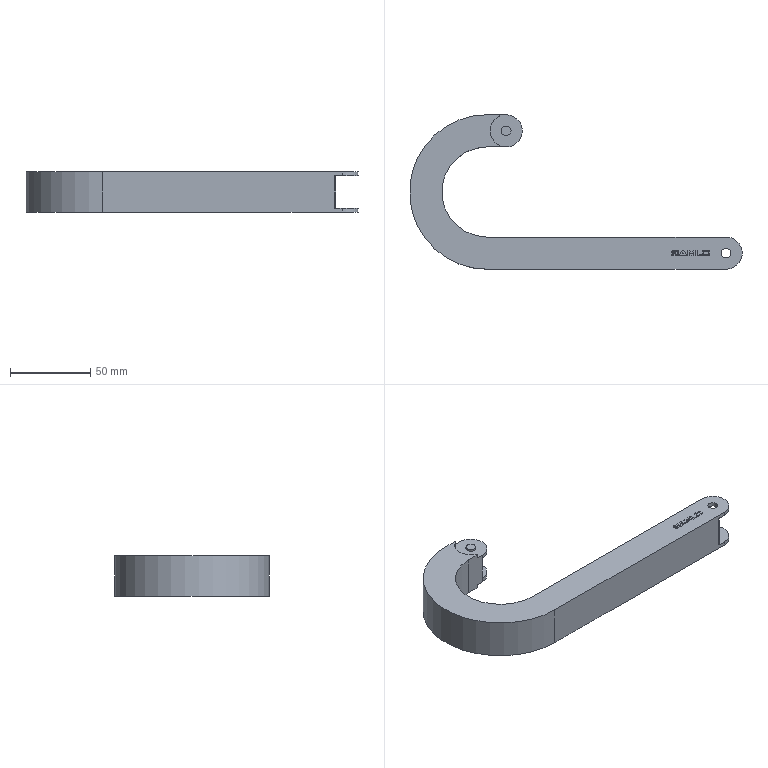Part | STEP file | TWD15-C15-R28-12(S0)_cable | 1 solid | 109 faces | box 206.68 x 96 x 25 mm | volume 76610 mm3 | plane 72 | cylinder 37 | commonest cylinder face diameters 6 x8 20 x7 1 x6 0.804 x4 1.704 x4 0.576 x2